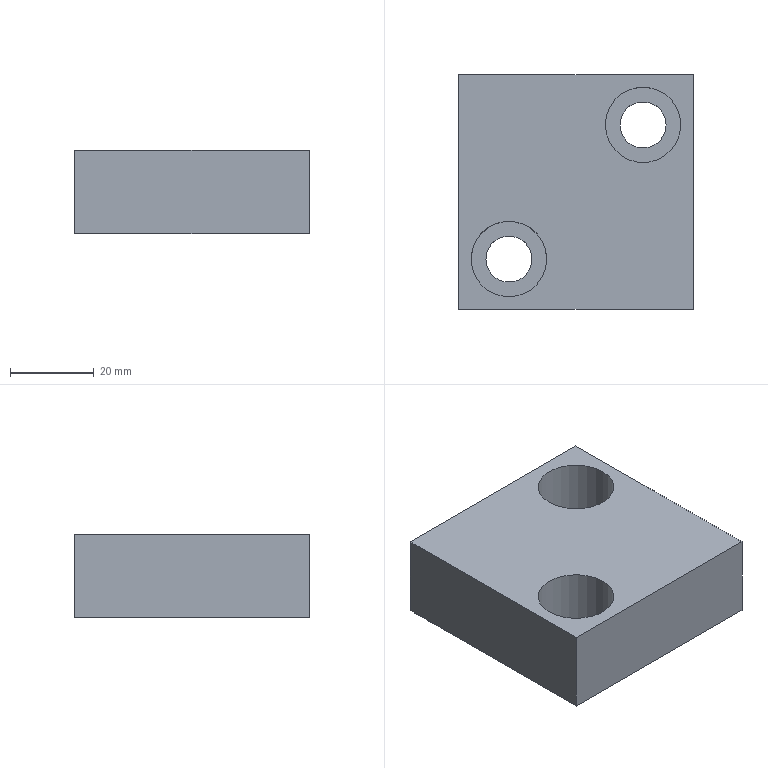Part | NX | features solid 2 | 1 solid | 12 faces | box 56 x 56 x 20 mm | volume 54773 mm3 | plane 8 | cylinder 4 | commonest cylinder face diameters 11 x2 18 x2
STEP:
#1=CARTESIAN_POINT('',(-1157.,462.,234.));
#2=VERTEX_POINT('',#1);
#3=CARTESIAN_POINT('',(-1157.,462.,254.));
#4=VERTEX_POINT('',#3);
#5=CARTESIAN_POINT('',(-1157.,462.,234.));
#6=DIRECTION('',(0.,0.,1.));
#7=VECTOR('',#6,1000.);
#8=LINE('',#5,#7);
#9=EDGE_CURVE('',#2,#4,#8,.T.);
#10=ORIENTED_EDGE('',*,*,#9,.F.);
#11=CARTESIAN_POINT('',(-1157.,518.,234.));
#12=VERTEX_POINT('',#11);
#13=CARTESIAN_POINT('',(-1157.,518.,234.));
#14=DIRECTION('',(0.,-1.,0.));
#15=VECTOR('',#14,1000.);
#16=LINE('',#13,#15);
#17=EDGE_CURVE('',#12,#2,#16,.T.);
#18=ORIENTED_EDGE('',*,*,#17,.F.);
#19=CARTESIAN_POINT('',(-1157.,518.,254.));
#20=VERTEX_POINT('',#19);
#21=CARTESIAN_POINT('',(-1157.,518.,234.));
#22=DIRECTION('',(0.,0.,1.));
#23=VECTOR('',#22,1000.);
#24=LINE('',#21,#23);
#25=EDGE_CURVE('',#12,#20,#24,.T.);
#26=ORIENTED_EDGE('',*,*,#25,.T.);
#27=CARTESIAN_POINT('',(-1157.,518.,254.));
#28=DIRECTION('',(0.,-1.,0.));
#29=VECTOR('',#28,1000.);
#30=LINE('',#27,#29);
#31=EDGE_CURVE('',#20,#4,#30,.T.);
#32=ORIENTED_EDGE('',*,*,#31,.T.);
#33=EDGE_LOOP('',(#10,#18,#26,#32));
#34=FACE_BOUND('',#33,.T.);
#35=CARTESIAN_POINT('',(-1157.,518.,234.));
#36=DIRECTION('',(1.,0.,0.));
#37=DIRECTION('',(0.,-1.,0.));
#38=AXIS2_PLACEMENT_3D('',#35,#36,#37);
#39=PLANE('',#38);
#40=ADVANCED_FACE('',(#34),#39,.T.);
#41=CARTESIAN_POINT('',(-1213.,462.,234.));
#42=VERTEX_POINT('',#41);
#43=CARTESIAN_POINT('',(-1213.,462.,254.));
#44=VERTEX_POINT('',#43);
#45=CARTESIAN_POINT('',(-1213.,462.,234.));
#46=DIRECTION('',(0.,0.,1.));
#47=VECTOR('',#46,1000.);
#48=LINE('',#45,#47);
#49=EDGE_CURVE('',#42,#44,#48,.T.);
#50=ORIENTED_EDGE('',*,*,#49,.F.);
#51=CARTESIAN_POINT('',(-1157.,462.,234.));
#52=DIRECTION('',(-1.,0.,0.));
#53=VECTOR('',#52,1000.);
#54=LINE('',#51,#53);
#55=EDGE_CURVE('',#2,#42,#54,.T.);
#56=ORIENTED_EDGE('',*,*,#55,.F.);
#57=ORIENTED_EDGE('',*,*,#9,.T.);
#58=CARTESIAN_POINT('',(-1157.,462.,254.));
#59=DIRECTION('',(-1.,0.,0.));
#60=VECTOR('',#59,1000.);
#61=LINE('',#58,#60);
#62=EDGE_CURVE('',#4,#44,#61,.T.);
#63=ORIENTED_EDGE('',*,*,#62,.T.);
#64=EDGE_LOOP('',(#50,#56,#57,#63));
#65=FACE_BOUND('',#64,.T.);
#66=CARTESIAN_POINT('',(-1157.,462.,234.));
#67=DIRECTION('',(0.,-1.,0.));
#68=DIRECTION('',(0.,0.,-1.));
#69=AXIS2_PLACEMENT_3D('',#66,#67,#68);
#70=PLANE('',#69);
#71=ADVANCED_FACE('',(#65),#70,.T.);
#72=CARTESIAN_POINT('',(-1213.,518.,234.));
#73=VERTEX_POINT('',#72);
#74=CARTESIAN_POINT('',(-1213.,518.,254.));
#75=VERTEX_POINT('',#74);
#76=CARTESIAN_POINT('',(-1213.,518.,234.));
#77=DIRECTION('',(0.,0.,1.));
#78=VECTOR('',#77,1000.);
#79=LINE('',#76,#78);
#80=EDGE_CURVE('',#73,#75,#79,.T.);
#81=ORIENTED_EDGE('',*,*,#80,.F.);
#82=CARTESIAN_POINT('',(-1213.,462.,234.));
#83=DIRECTION('',(0.,1.,0.));
#84=VECTOR('',#83,1000.);
#85=LINE('',#82,#84);
#86=EDGE_CURVE('',#42,#73,#85,.T.);
#87=ORIENTED_EDGE('',*,*,#86,.F.);
#88=ORIENTED_EDGE('',*,*,#49,.T.);
#89=CARTESIAN_POINT('',(-1213.,462.,254.));
#90=DIRECTION('',(0.,1.,0.));
#91=VECTOR('',#90,1000.);
#92=LINE('',#89,#91);
#93=EDGE_CURVE('',#44,#75,#92,.T.);
#94=ORIENTED_EDGE('',*,*,#93,.T.);
#95=EDGE_LOOP('',(#81,#87,#88,#94));
#96=FACE_BOUND('',#95,.T.);
#97=CARTESIAN_POINT('',(-1213.,462.,234.));
#98=DIRECTION('',(-1.,0.,0.));
#99=DIRECTION('',(0.,0.,-1.));
#100=AXIS2_PLACEMENT_3D('',#97,#98,#99);
#101=PLANE('',#100);
#102=ADVANCED_FACE('',(#96),#101,.T.);
#103=CARTESIAN_POINT('',(-1163.5,506.,241.));
#104=VERTEX_POINT('',#103);
#105=CARTESIAN_POINT('',(-1169.,506.,241.));
#106=DIRECTION('',(0.,0.,1.));
#107=DIRECTION('',(1.,0.,0.));
#108=AXIS2_PLACEMENT_3D('',#105,#106,#107);
#109=CIRCLE('',#108,5.5);
#110=EDGE_CURVE('',#104,#104,#109,.F.);
#111=ORIENTED_EDGE('',*,*,#110,.F.);
#112=EDGE_LOOP('',(#111));
#113=FACE_BOUND('',#112,.T.);
#114=CARTESIAN_POINT('',(-1174.5,506.,234.));
#115=VERTEX_POINT('',#114);
#116=CARTESIAN_POINT('',(-1169.,506.,234.));
#117=DIRECTION('',(0.,0.,-1.));
#118=DIRECTION('',(-1.,0.,0.));
#119=AXIS2_PLACEMENT_3D('',#116,#117,#118);
#120=CIRCLE('',#119,5.5);
#121=EDGE_CURVE('',#115,#115,#120,.T.);
#122=ORIENTED_EDGE('',*,*,#121,.T.);
#123=EDGE_LOOP('',(#122));
#124=FACE_BOUND('',#123,.T.);
#125=CARTESIAN_POINT('',(-1169.,506.,234.));
#126=DIRECTION('',(0.,0.,1.));
#127=DIRECTION('',(-1.,0.,0.));
#128=AXIS2_PLACEMENT_3D('',#125,#126,#127);
#129=CYLINDRICAL_SURFACE('',#128,5.5);
#130=ADVANCED_FACE('',(#113,#124),#129,.F.);
#131=CARTESIAN_POINT('',(-1195.5,474.,241.));
#132=VERTEX_POINT('',#131);
#133=CARTESIAN_POINT('',(-1201.,474.,241.));
#134=DIRECTION('',(0.,0.,1.));
#135=DIRECTION('',(1.,0.,0.));
#136=AXIS2_PLACEMENT_3D('',#133,#134,#135);
#137=CIRCLE('',#136,5.5);
#138=EDGE_CURVE('',#132,#132,#137,.F.);
#139=ORIENTED_EDGE('',*,*,#138,.F.);
#140=EDGE_LOOP('',(#139));
#141=FACE_BOUND('',#140,.T.);
#142=CARTESIAN_POINT('',(-1206.5,474.,234.));
#143=VERTEX_POINT('',#142);
#144=CARTESIAN_POINT('',(-1201.,474.,234.));
#145=DIRECTION('',(0.,0.,-1.));
#146=DIRECTION('',(-1.,0.,0.));
#147=AXIS2_PLACEMENT_3D('',#144,#145,#146);
#148=CIRCLE('',#147,5.5);
#149=EDGE_CURVE('',#143,#143,#148,.T.);
#150=ORIENTED_EDGE('',*,*,#149,.T.);
#151=EDGE_LOOP('',(#150));
#152=FACE_BOUND('',#151,.T.);
#153=CARTESIAN_POINT('',(-1201.,474.,234.));
#154=DIRECTION('',(0.,0.,1.));
#155=DIRECTION('',(-1.,0.,0.));
#156=AXIS2_PLACEMENT_3D('',#153,#154,#155);
#157=CYLINDRICAL_SURFACE('',#156,5.5);
#158=ADVANCED_FACE('',(#141,#152),#157,.F.);
#159=CARTESIAN_POINT('',(-1213.,518.,234.));
#160=DIRECTION('',(1.,0.,0.));
#161=VECTOR('',#160,1000.);
#162=LINE('',#159,#161);
#163=EDGE_CURVE('',#73,#12,#162,.T.);
#164=ORIENTED_EDGE('',*,*,#163,.F.);
#165=ORIENTED_EDGE('',*,*,#80,.T.);
#166=CARTESIAN_POINT('',(-1213.,518.,254.));
#167=DIRECTION('',(1.,0.,0.));
#168=VECTOR('',#167,1000.);
#169=LINE('',#166,#168);
#170=EDGE_CURVE('',#75,#20,#169,.T.);
#171=ORIENTED_EDGE('',*,*,#170,.T.);
#172=ORIENTED_EDGE('',*,*,#25,.F.);
#173=EDGE_LOOP('',(#164,#165,#171,#172));
#174=FACE_BOUND('',#173,.T.);
#175=CARTESIAN_POINT('',(-1213.,518.,234.));
#176=DIRECTION('',(0.,1.,0.));
#177=DIRECTION('',(1.,0.,0.));
#178=AXIS2_PLACEMENT_3D('',#175,#176,#177);
#179=PLANE('',#178);
#180=ADVANCED_FACE('',(#174),#179,.T.);
#181=ORIENTED_EDGE('',*,*,#149,.F.);
#182=EDGE_LOOP('',(#181));
#183=FACE_BOUND('',#182,.T.);
#184=ORIENTED_EDGE('',*,*,#121,.F.);
#185=EDGE_LOOP('',(#184));
#186=FACE_BOUND('',#185,.T.);
#187=ORIENTED_EDGE('',*,*,#17,.T.);
#188=ORIENTED_EDGE('',*,*,#55,.T.);
#189=ORIENTED_EDGE('',*,*,#86,.T.);
#190=ORIENTED_EDGE('',*,*,#163,.T.);
#191=EDGE_LOOP('',(#187,#188,#189,#190));
#192=FACE_BOUND('',#191,.T.);
#193=CARTESIAN_POINT('',(-1157.,518.,234.));
#194=DIRECTION('',(0.,0.,-1.));
#195=DIRECTION('',(1.,0.,0.));
#196=AXIS2_PLACEMENT_3D('',#193,#194,#195);
#197=PLANE('',#196);
#198=ADVANCED_FACE('',(#183,#186,#192),#197,.T.);
#199=CARTESIAN_POINT('',(-1192.,474.,254.));
#200=VERTEX_POINT('',#199);
#201=CARTESIAN_POINT('',(-1201.,474.,254.));
#202=DIRECTION('',(0.,0.,1.));
#203=DIRECTION('',(1.,0.,0.));
#204=AXIS2_PLACEMENT_3D('',#201,#202,#203);
#205=CIRCLE('',#204,9.);
#206=EDGE_CURVE('',#200,#200,#205,.T.);
#207=ORIENTED_EDGE('',*,*,#206,.F.);
#208=EDGE_LOOP('',(#207));
#209=FACE_BOUND('',#208,.T.);
#210=CARTESIAN_POINT('',(-1160.,506.,254.));
#211=VERTEX_POINT('',#210);
#212=CARTESIAN_POINT('',(-1169.,506.,254.));
#213=DIRECTION('',(0.,0.,1.));
#214=DIRECTION('',(1.,0.,0.));
#215=AXIS2_PLACEMENT_3D('',#212,#213,#214);
#216=CIRCLE('',#215,9.);
#217=EDGE_CURVE('',#211,#211,#216,.T.);
#218=ORIENTED_EDGE('',*,*,#217,.F.);
#219=EDGE_LOOP('',(#218));
#220=FACE_BOUND('',#219,.T.);
#221=ORIENTED_EDGE('',*,*,#31,.F.);
#222=ORIENTED_EDGE('',*,*,#170,.F.);
#223=ORIENTED_EDGE('',*,*,#93,.F.);
#224=ORIENTED_EDGE('',*,*,#62,.F.);
#225=EDGE_LOOP('',(#221,#222,#223,#224));
#226=FACE_BOUND('',#225,.T.);
#227=CARTESIAN_POINT('',(-1157.,518.,254.));
#228=DIRECTION('',(0.,0.,-1.));
#229=DIRECTION('',(1.,0.,0.));
#230=AXIS2_PLACEMENT_3D('',#227,#228,#229);
#231=PLANE('',#230);
#232=ADVANCED_FACE('',(#209,#220,#226),#231,.F.);
#233=CARTESIAN_POINT('',(-1160.,506.,241.));
#234=VERTEX_POINT('',#233);
#235=CARTESIAN_POINT('',(-1169.,506.,241.));
#236=DIRECTION('',(0.,0.,1.));
#237=DIRECTION('',(1.,0.,0.));
#238=AXIS2_PLACEMENT_3D('',#235,#236,#237);
#239=CIRCLE('',#238,9.);
#240=EDGE_CURVE('',#234,#234,#239,.T.);
#241=ORIENTED_EDGE('',*,*,#240,.T.);
#242=EDGE_LOOP('',(#241));
#243=FACE_BOUND('',#242,.T.);
#244=ORIENTED_EDGE('',*,*,#110,.T.);
#245=EDGE_LOOP('',(#244));
#246=FACE_BOUND('',#245,.T.);
#247=CARTESIAN_POINT('',(-1169.,506.,241.));
#248=DIRECTION('',(0.,0.,-1.));
#249=DIRECTION('',(1.,0.,0.));
#250=AXIS2_PLACEMENT_3D('',#247,#248,#249);
#251=PLANE('',#250);
#252=ADVANCED_FACE('',(#243,#246),#251,.F.);
#253=ORIENTED_EDGE('',*,*,#240,.F.);
#254=EDGE_LOOP('',(#253));
#255=FACE_BOUND('',#254,.T.);
#256=ORIENTED_EDGE('',*,*,#217,.T.);
#257=EDGE_LOOP('',(#256));
#258=FACE_BOUND('',#257,.T.);
#259=CARTESIAN_POINT('',(-1169.,506.,254.));
#260=DIRECTION('',(0.,0.,-1.));
#261=DIRECTION('',(1.,0.,0.));
#262=AXIS2_PLACEMENT_3D('',#259,#260,#261);
#263=CYLINDRICAL_SURFACE('',#262,9.);
#264=ADVANCED_FACE('',(#255,#258),#263,.F.);
#265=CARTESIAN_POINT('',(-1192.,474.,241.));
#266=VERTEX_POINT('',#265);
#267=CARTESIAN_POINT('',(-1201.,474.,241.));
#268=DIRECTION('',(0.,0.,1.));
#269=DIRECTION('',(1.,0.,0.));
#270=AXIS2_PLACEMENT_3D('',#267,#268,#269);
#271=CIRCLE('',#270,9.);
#272=EDGE_CURVE('',#266,#266,#271,.T.);
#273=ORIENTED_EDGE('',*,*,#272,.T.);
#274=EDGE_LOOP('',(#273));
#275=FACE_BOUND('',#274,.T.);
#276=ORIENTED_EDGE('',*,*,#138,.T.);
#277=EDGE_LOOP('',(#276));
#278=FACE_BOUND('',#277,.T.);
#279=CARTESIAN_POINT('',(-1201.,474.,241.));
#280=DIRECTION('',(0.,0.,-1.));
#281=DIRECTION('',(1.,0.,0.));
#282=AXIS2_PLACEMENT_3D('',#279,#280,#281);
#283=PLANE('',#282);
#284=ADVANCED_FACE('',(#275,#278),#283,.F.);
#285=ORIENTED_EDGE('',*,*,#272,.F.);
#286=EDGE_LOOP('',(#285));
#287=FACE_BOUND('',#286,.T.);
#288=ORIENTED_EDGE('',*,*,#206,.T.);
#289=EDGE_LOOP('',(#288));
#290=FACE_BOUND('',#289,.T.);
#291=CARTESIAN_POINT('',(-1201.,474.,254.));
#292=DIRECTION('',(0.,0.,-1.));
#293=DIRECTION('',(1.,0.,0.));
#294=AXIS2_PLACEMENT_3D('',#291,#292,#293);
#295=CYLINDRICAL_SURFACE('',#294,9.);
#296=ADVANCED_FACE('',(#287,#290),#295,.F.);
#297=CLOSED_SHELL('',(#40,#71,#102,#130,#158,#180,#198,#232,#252,#264,#284,#296));
#298=MANIFOLD_SOLID_BREP('',#297);
#299=(LENGTH_UNIT()NAMED_UNIT(*)SI_UNIT(.MILLI.,.METRE.));
#300=UNCERTAINTY_MEASURE_WITH_UNIT(LENGTH_MEASURE(0.00001),#299,'','');
#301=(NAMED_UNIT(*)PLANE_ANGLE_UNIT()SI_UNIT($,.RADIAN.));
#302=(NAMED_UNIT(*)SI_UNIT($,.STERADIAN.)SOLID_ANGLE_UNIT());
#303=(GEOMETRIC_REPRESENTATION_CONTEXT(3)GLOBAL_UNCERTAINTY_ASSIGNED_CONTEXT((#300))GLOBAL_UNIT_ASSIGNED_CONTEXT((#299,#301,#302))REPRESENTATION_CONTEXT('',''));
#304=ADVANCED_BREP_SHAPE_REPRESENTATION('',(#298),#303);